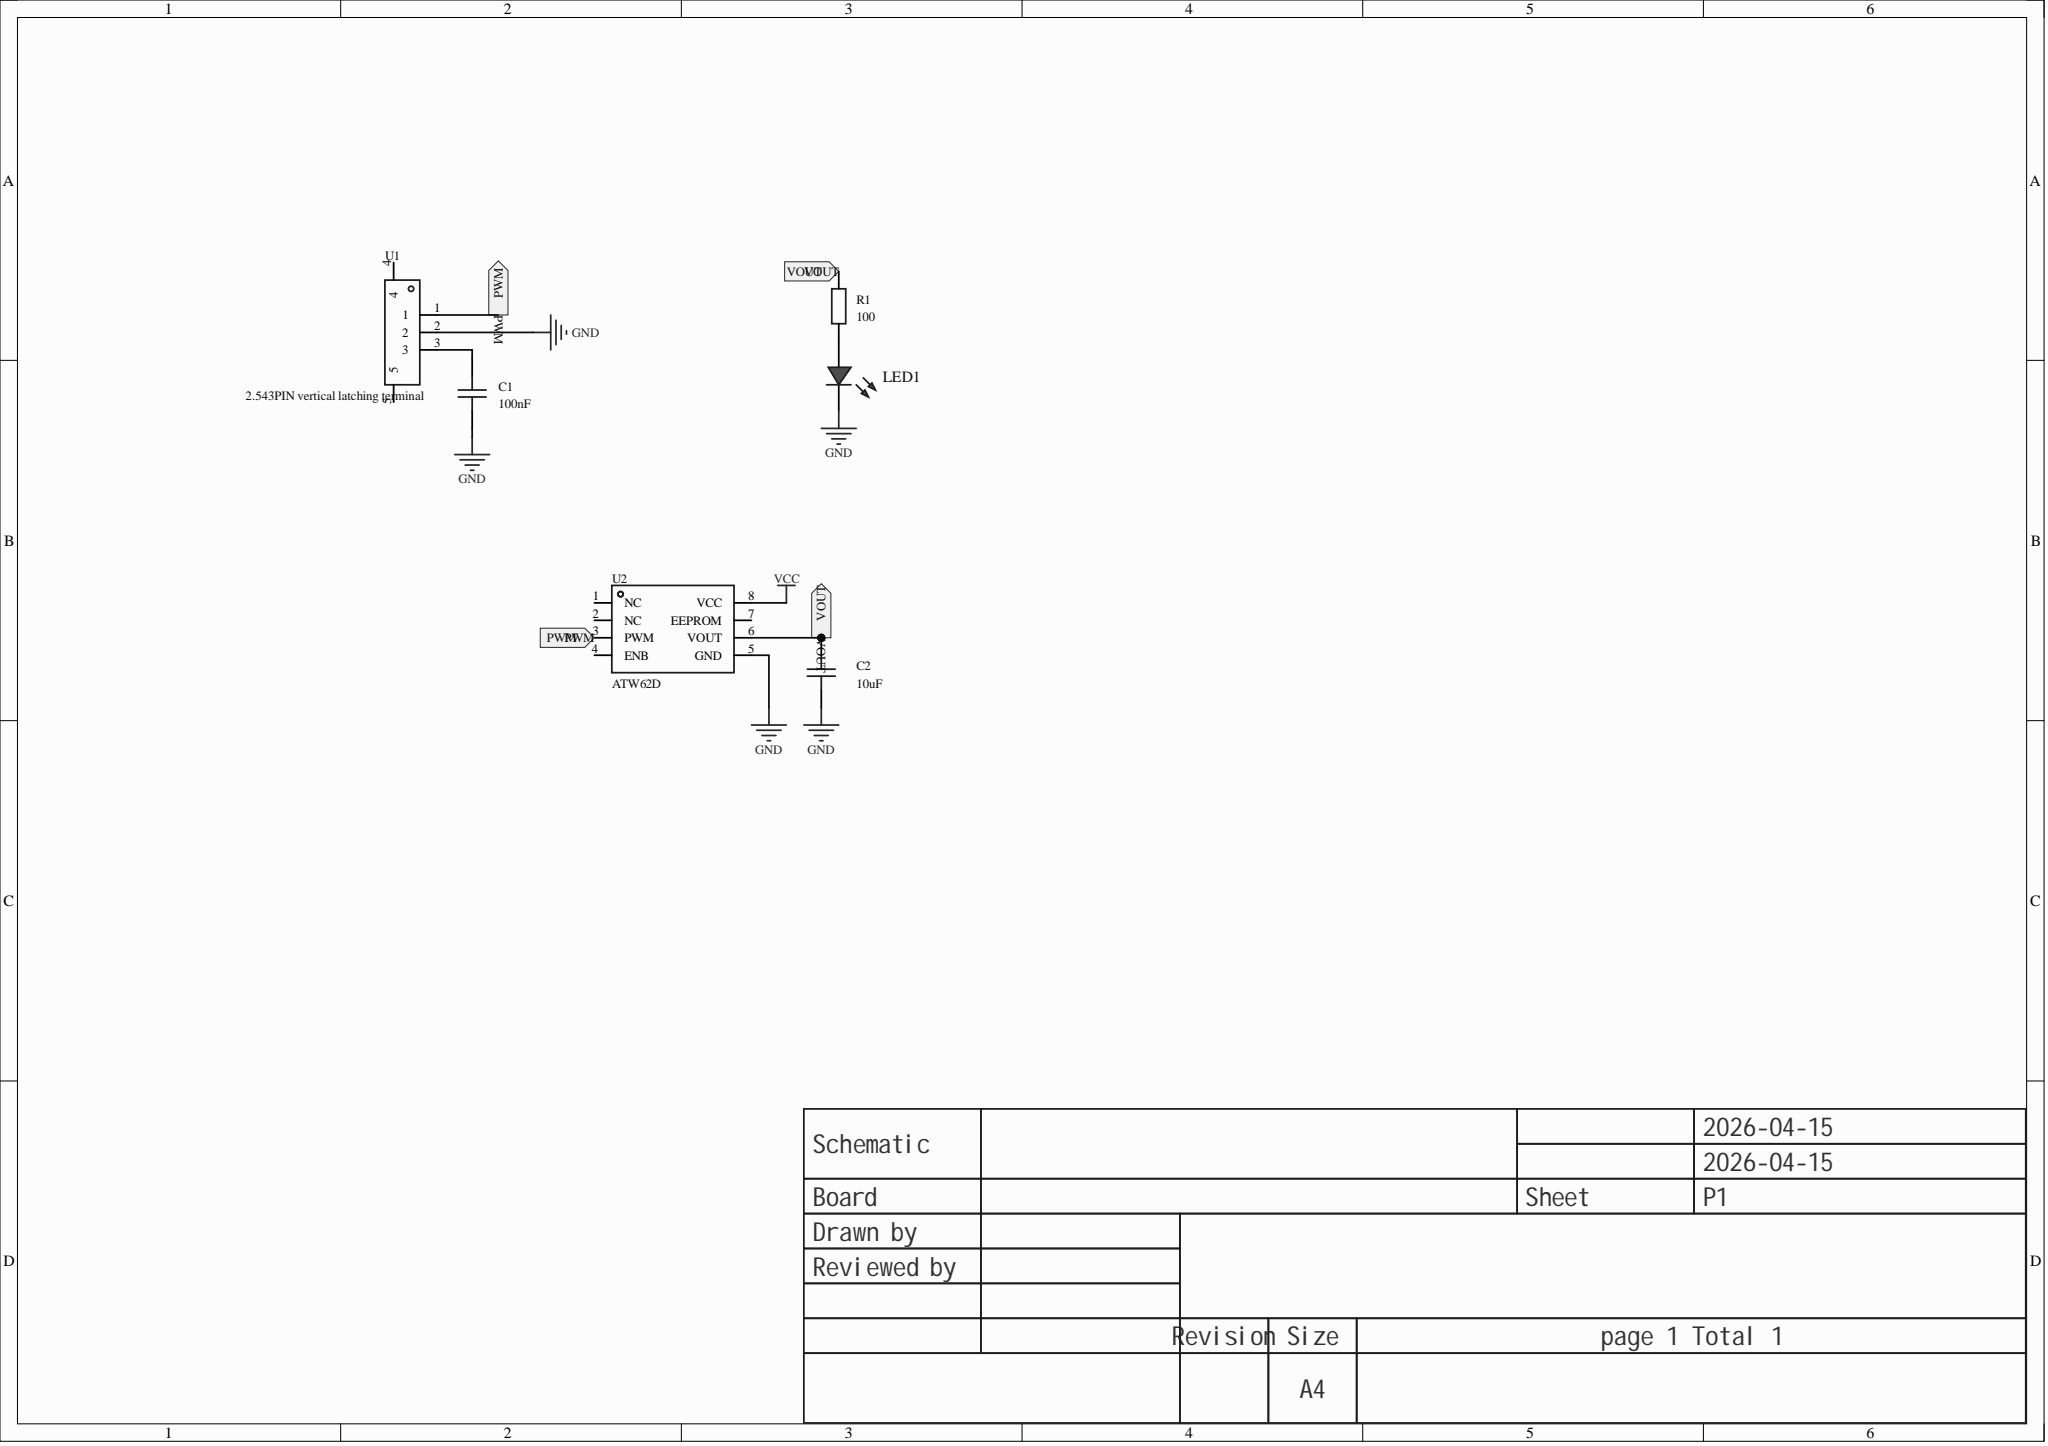Circuit board | Altium Designer | 6 parts | 5 nets
Bill of materials:
Comment,Description,Designator,Footprint,LibRef,Quantity
"100nF","","C1","C0603","CAP_0603","1"
"10uF","","C2","C0603","CAP_0603","1"
"","","LED1","LED_0603","LED_0603-R","1"
"100","","R1","R0603","Res_0603","1"
"2.543PIN vertical latching terminal","","U1","CONN-SMD_3P-P2.54_C9900012759","2.543PIN立式带扣端子","1"
"ATW62D","","U2","SOP-8_L4.9-W3.9-P1.27-LS6.0-TL","ATW62D","1"
Netlist (Protel format):
[
C1
C0603
100nF



]
[
C2
C0603
10uF



]
[
LED1
LED_0603




]
[
R1
R0603
100



]
[
U1
CONN-SMD_3P-P2.54_C9900012759
2.543PIN vertical latching terminal



]
[
U2
SOP-8_L4.9-W3.9-P1.27-LS6.0-TL
ATW62D



]
(
VOUT
C2-2
R1-2
U2-6
)
(
PWM
U1-1
U2-3
)
(
NetLED1_2
LED1-2
R1-1
)
(
NetC1_2
C1-2
U1-3
)
(
GND
C1-1
C2-1
LED1-1
U1-2
U2-5
)